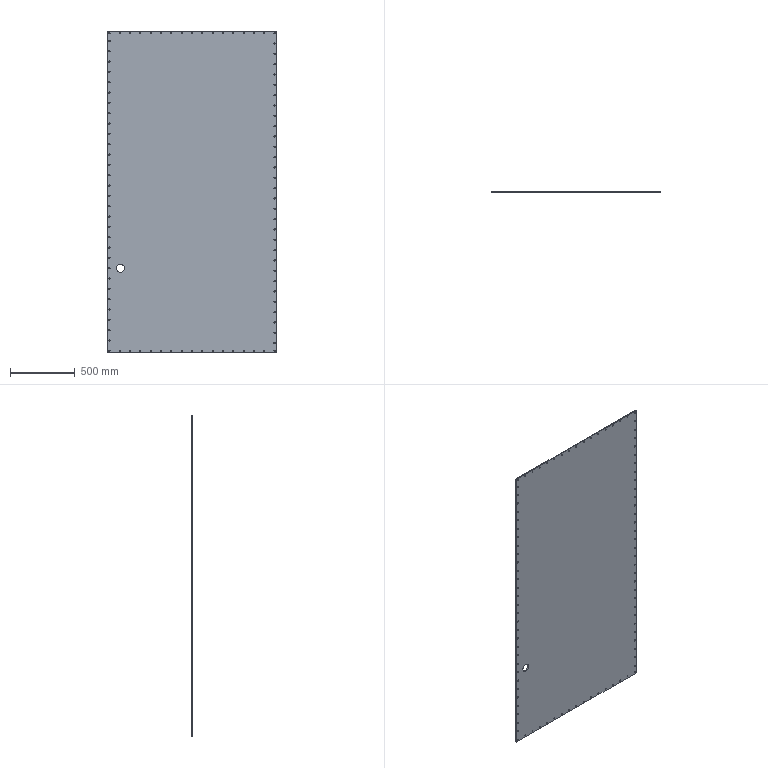Part | SolidWorks | features CirPattern 2, HoleWzd 2, LPattern 2, FlatPattern 1, ICE 1, RefAxis 1, SMBaseFlange 1, SheetMetal 1 | 1 solid | 196 faces | box 1310 x 8 x 2490 mm | volume 26011985 mm3 | cylinder 190 | plane 6 | commonest cylinder face diameters 10 x188 62 x2